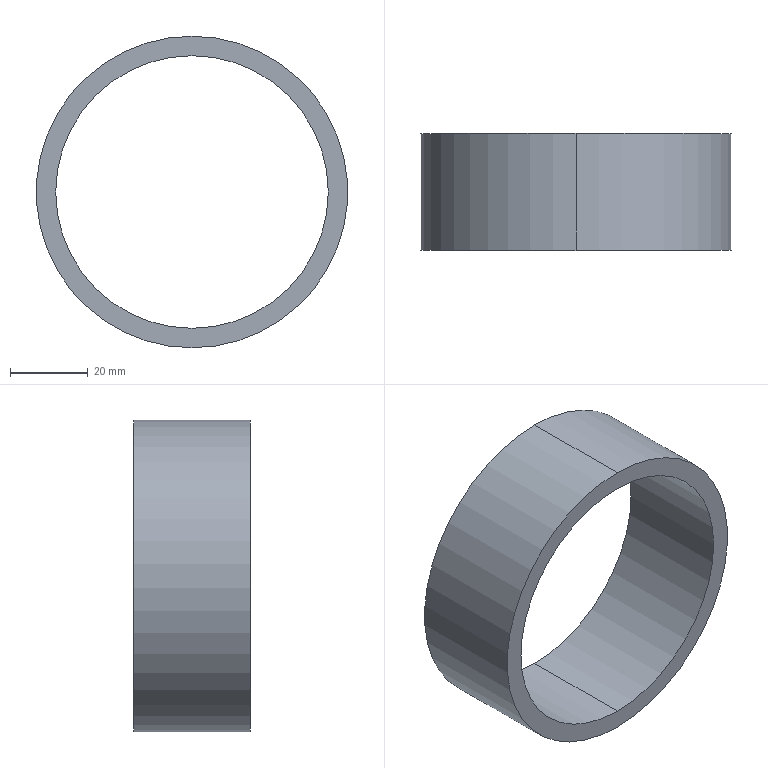Part | SolidWorks | features BaseBody 1 | 1 solid | 6 faces | box 80 x 30 x 80 mm | volume 35343 mm3 | cylinder 4 | plane 2 | commonest cylinder face diameters 70 x2 80 x2
STEP:
#1=CARTESIAN_POINT('',(0.,30.,-35.));
#2=VERTEX_POINT('',#1);
#3=CARTESIAN_POINT('',(0.,30.,35.));
#4=VERTEX_POINT('',#3);
#5=CARTESIAN_POINT('',(0.,30.,0.));
#6=DIRECTION('',(0.,1.,0.));
#7=DIRECTION('',(0.,0.,1.));
#8=AXIS2_PLACEMENT_3D('',#5,#6,#7);
#9=CIRCLE('',#8,35.);
#10=EDGE_CURVE('',#2,#4,#9,.T.);
#11=ORIENTED_EDGE('',*,*,#10,.T.);
#12=CARTESIAN_POINT('',(0.,0.,35.));
#13=VERTEX_POINT('',#12);
#14=CARTESIAN_POINT('',(0.,30.,35.));
#15=DIRECTION('',(0.,-1.,0.));
#16=VECTOR('',#15,1000.);
#17=LINE('',#14,#16);
#18=EDGE_CURVE('',#4,#13,#17,.T.);
#19=ORIENTED_EDGE('',*,*,#18,.T.);
#20=CARTESIAN_POINT('',(0.,0.,-35.));
#21=VERTEX_POINT('',#20);
#22=CARTESIAN_POINT('',(0.,0.,0.));
#23=DIRECTION('',(0.,1.,0.));
#24=DIRECTION('',(0.,0.,1.));
#25=AXIS2_PLACEMENT_3D('',#22,#23,#24);
#26=CIRCLE('',#25,35.);
#27=EDGE_CURVE('',#21,#13,#26,.T.);
#28=ORIENTED_EDGE('',*,*,#27,.F.);
#29=CARTESIAN_POINT('',(0.,30.,-35.));
#30=DIRECTION('',(0.,-1.,0.));
#31=VECTOR('',#30,1000.);
#32=LINE('',#29,#31);
#33=EDGE_CURVE('',#2,#21,#32,.T.);
#34=ORIENTED_EDGE('',*,*,#33,.F.);
#35=EDGE_LOOP('',(#11,#19,#28,#34));
#36=FACE_OUTER_BOUND('',#35,.T.);
#37=CARTESIAN_POINT('',(0.,30.,0.));
#38=DIRECTION('',(0.,-1.,0.));
#39=DIRECTION('',(0.,0.,-1.));
#40=AXIS2_PLACEMENT_3D('',#37,#38,#39);
#41=CYLINDRICAL_SURFACE('',#40,35.);
#42=ADVANCED_FACE('',(#36),#41,.F.);
#43=CARTESIAN_POINT('',(0.,30.,40.));
#44=VERTEX_POINT('',#43);
#45=CARTESIAN_POINT('',(0.,30.,-40.));
#46=VERTEX_POINT('',#45);
#47=CARTESIAN_POINT('',(0.,30.,0.));
#48=DIRECTION('',(0.,1.,0.));
#49=DIRECTION('',(0.,0.,1.));
#50=AXIS2_PLACEMENT_3D('',#47,#48,#49);
#51=CIRCLE('',#50,40.);
#52=EDGE_CURVE('',#44,#46,#51,.T.);
#53=ORIENTED_EDGE('',*,*,#52,.F.);
#54=CARTESIAN_POINT('',(0.,0.,40.));
#55=VERTEX_POINT('',#54);
#56=CARTESIAN_POINT('',(0.,30.,40.));
#57=DIRECTION('',(0.,-1.,0.));
#58=VECTOR('',#57,1000.);
#59=LINE('',#56,#58);
#60=EDGE_CURVE('',#44,#55,#59,.T.);
#61=ORIENTED_EDGE('',*,*,#60,.T.);
#62=CARTESIAN_POINT('',(0.,0.,-40.));
#63=VERTEX_POINT('',#62);
#64=CARTESIAN_POINT('',(0.,0.,0.));
#65=DIRECTION('',(0.,1.,0.));
#66=DIRECTION('',(0.,0.,1.));
#67=AXIS2_PLACEMENT_3D('',#64,#65,#66);
#68=CIRCLE('',#67,40.);
#69=EDGE_CURVE('',#55,#63,#68,.T.);
#70=ORIENTED_EDGE('',*,*,#69,.T.);
#71=CARTESIAN_POINT('',(0.,30.,-40.));
#72=DIRECTION('',(0.,-1.,0.));
#73=VECTOR('',#72,1000.);
#74=LINE('',#71,#73);
#75=EDGE_CURVE('',#46,#63,#74,.T.);
#76=ORIENTED_EDGE('',*,*,#75,.F.);
#77=EDGE_LOOP('',(#53,#61,#70,#76));
#78=FACE_OUTER_BOUND('',#77,.T.);
#79=CARTESIAN_POINT('',(0.,30.,0.));
#80=DIRECTION('',(0.,-1.,0.));
#81=DIRECTION('',(0.,0.,-1.));
#82=AXIS2_PLACEMENT_3D('',#79,#80,#81);
#83=CYLINDRICAL_SURFACE('',#82,40.);
#84=ADVANCED_FACE('',(#78),#83,.T.);
#85=CARTESIAN_POINT('',(0.,30.,0.));
#86=DIRECTION('',(0.,1.,0.));
#87=DIRECTION('',(0.,0.,1.));
#88=AXIS2_PLACEMENT_3D('',#85,#86,#87);
#89=CIRCLE('',#88,40.);
#90=EDGE_CURVE('',#46,#44,#89,.T.);
#91=ORIENTED_EDGE('',*,*,#90,.T.);
#92=ORIENTED_EDGE('',*,*,#52,.T.);
#93=EDGE_LOOP('',(#91,#92));
#94=FACE_OUTER_BOUND('',#93,.T.);
#95=ORIENTED_EDGE('',*,*,#10,.F.);
#96=CARTESIAN_POINT('',(0.,30.,0.));
#97=DIRECTION('',(0.,1.,0.));
#98=DIRECTION('',(0.,0.,1.));
#99=AXIS2_PLACEMENT_3D('',#96,#97,#98);
#100=CIRCLE('',#99,35.);
#101=EDGE_CURVE('',#4,#2,#100,.T.);
#102=ORIENTED_EDGE('',*,*,#101,.F.);
#103=EDGE_LOOP('',(#95,#102));
#104=FACE_BOUND('',#103,.T.);
#105=CARTESIAN_POINT('',(0.,30.,0.));
#106=DIRECTION('',(0.,1.,0.));
#107=DIRECTION('',(0.,0.,1.));
#108=AXIS2_PLACEMENT_3D('',#105,#106,#107);
#109=PLANE('',#108);
#110=ADVANCED_FACE('',(#94,#104),#109,.T.);
#111=CARTESIAN_POINT('',(0.,0.,0.));
#112=DIRECTION('',(0.,1.,0.));
#113=DIRECTION('',(0.,0.,1.));
#114=AXIS2_PLACEMENT_3D('',#111,#112,#113);
#115=CIRCLE('',#114,40.);
#116=EDGE_CURVE('',#63,#55,#115,.T.);
#117=ORIENTED_EDGE('',*,*,#116,.F.);
#118=ORIENTED_EDGE('',*,*,#69,.F.);
#119=EDGE_LOOP('',(#117,#118));
#120=FACE_OUTER_BOUND('',#119,.T.);
#121=ORIENTED_EDGE('',*,*,#27,.T.);
#122=CARTESIAN_POINT('',(0.,0.,0.));
#123=DIRECTION('',(0.,1.,0.));
#124=DIRECTION('',(0.,0.,1.));
#125=AXIS2_PLACEMENT_3D('',#122,#123,#124);
#126=CIRCLE('',#125,35.);
#127=EDGE_CURVE('',#13,#21,#126,.T.);
#128=ORIENTED_EDGE('',*,*,#127,.T.);
#129=EDGE_LOOP('',(#121,#128));
#130=FACE_BOUND('',#129,.T.);
#131=CARTESIAN_POINT('',(0.,0.,0.));
#132=DIRECTION('',(0.,1.,0.));
#133=DIRECTION('',(0.,0.,1.));
#134=AXIS2_PLACEMENT_3D('',#131,#132,#133);
#135=PLANE('',#134);
#136=ADVANCED_FACE('',(#120,#130),#135,.F.);
#137=ORIENTED_EDGE('',*,*,#60,.F.);
#138=ORIENTED_EDGE('',*,*,#90,.F.);
#139=ORIENTED_EDGE('',*,*,#75,.T.);
#140=ORIENTED_EDGE('',*,*,#116,.T.);
#141=EDGE_LOOP('',(#137,#138,#139,#140));
#142=FACE_OUTER_BOUND('',#141,.T.);
#143=CARTESIAN_POINT('',(0.,30.,0.));
#144=DIRECTION('',(0.,-1.,0.));
#145=DIRECTION('',(0.,0.,-1.));
#146=AXIS2_PLACEMENT_3D('',#143,#144,#145);
#147=CYLINDRICAL_SURFACE('',#146,40.);
#148=ADVANCED_FACE('',(#142),#147,.T.);
#149=ORIENTED_EDGE('',*,*,#18,.F.);
#150=ORIENTED_EDGE('',*,*,#101,.T.);
#151=ORIENTED_EDGE('',*,*,#33,.T.);
#152=ORIENTED_EDGE('',*,*,#127,.F.);
#153=EDGE_LOOP('',(#149,#150,#151,#152));
#154=FACE_OUTER_BOUND('',#153,.T.);
#155=CARTESIAN_POINT('',(0.,30.,0.));
#156=DIRECTION('',(0.,-1.,0.));
#157=DIRECTION('',(0.,0.,-1.));
#158=AXIS2_PLACEMENT_3D('',#155,#156,#157);
#159=CYLINDRICAL_SURFACE('',#158,35.);
#160=ADVANCED_FACE('',(#154),#159,.F.);
#161=CLOSED_SHELL('',(#42,#84,#110,#136,#148,#160));
#162=MANIFOLD_SOLID_BREP('',#161);
#163=CARTESIAN_POINT('',(0.,0.,0.));
#164=DIRECTION('',(0.,0.,1.));
#165=DIRECTION('',(1.,0.,0.));
#166=AXIS2_PLACEMENT_3D('',#163,#164,#165);
#167=(LENGTH_UNIT()NAMED_UNIT(*)SI_UNIT(.MILLI.,.METRE.));
#168=UNCERTAINTY_MEASURE_WITH_UNIT(LENGTH_MEASURE(0.00001),#167,'','');
#169=(NAMED_UNIT(*)PLANE_ANGLE_UNIT()SI_UNIT($,.RADIAN.));
#170=(NAMED_UNIT(*)SI_UNIT($,.STERADIAN.)SOLID_ANGLE_UNIT());
#171=(GEOMETRIC_REPRESENTATION_CONTEXT(3)GLOBAL_UNCERTAINTY_ASSIGNED_CONTEXT((#168))GLOBAL_UNIT_ASSIGNED_CONTEXT((#167,#169,#170))REPRESENTATION_CONTEXT('',''));
#172=ADVANCED_BREP_SHAPE_REPRESENTATION('',(#162,#166),#171);